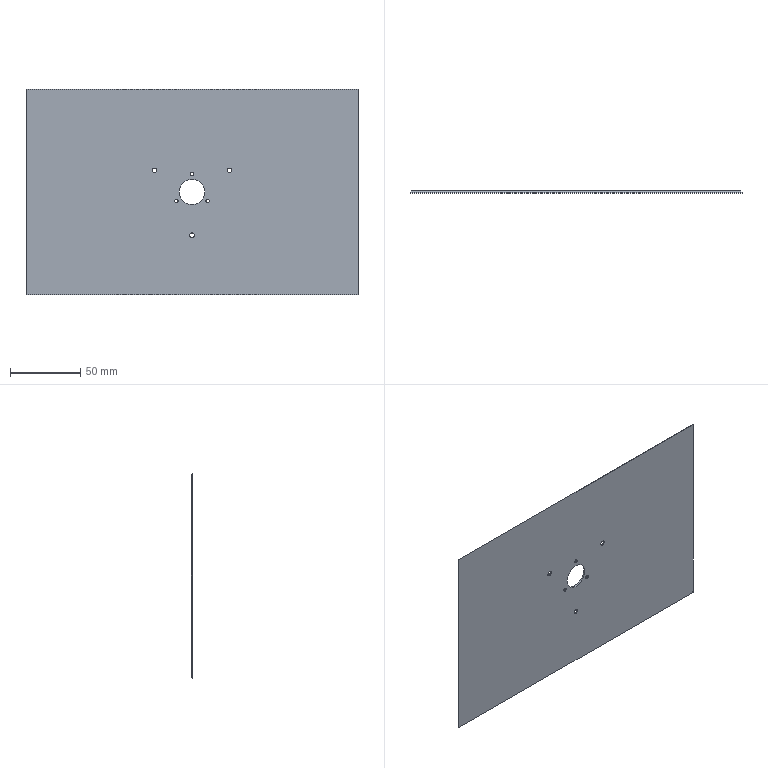Part | NX | 1 solid | 32 faces | box 236.4 x 1.2 x 146.4 mm | volume 40622 mm3 | cylinder 14 | cone 12 | plane 6 | commonest cylinder face diameters 2.5 x6 3.3 x6 18 x2
STEP:
#1=CARTESIAN_POINT('',(-117.,110.,72.));
#2=VERTEX_POINT('',#1);
#3=CARTESIAN_POINT('',(-117.,110.,-72.));
#4=VERTEX_POINT('',#3);
#5=CARTESIAN_POINT('',(-117.,110.,0.));
#6=DIRECTION('',(0.,0.,-1.));
#7=VECTOR('',#6,1000.);
#8=LINE('',#5,#7);
#9=EDGE_CURVE('',#2,#4,#8,.T.);
#10=ORIENTED_EDGE('',*,*,#9,.F.);
#11=CARTESIAN_POINT('',(117.,110.,72.));
#12=VERTEX_POINT('',#11);
#13=CARTESIAN_POINT('',(0.,110.,72.));
#14=DIRECTION('',(-1.,0.,0.));
#15=VECTOR('',#14,1000.);
#16=LINE('',#13,#15);
#17=EDGE_CURVE('',#12,#2,#16,.T.);
#18=ORIENTED_EDGE('',*,*,#17,.F.);
#19=CARTESIAN_POINT('',(117.,110.,-72.));
#20=VERTEX_POINT('',#19);
#21=CARTESIAN_POINT('',(117.,110.,0.));
#22=DIRECTION('',(0.,0.,1.));
#23=VECTOR('',#22,1000.);
#24=LINE('',#21,#23);
#25=EDGE_CURVE('',#20,#12,#24,.T.);
#26=ORIENTED_EDGE('',*,*,#25,.F.);
#27=CARTESIAN_POINT('',(0.,110.,-72.));
#28=DIRECTION('',(-1.,0.,0.));
#29=VECTOR('',#28,1000.);
#30=LINE('',#27,#29);
#31=EDGE_CURVE('',#20,#4,#30,.T.);
#32=ORIENTED_EDGE('',*,*,#31,.T.);
#33=EDGE_LOOP('',(#10,#18,#26,#32));
#34=FACE_BOUND('',#33,.T.);
#35=CARTESIAN_POINT('',(-28.945,110.,15.375));
#36=VERTEX_POINT('',#35);
#37=CARTESIAN_POINT('',(-24.315,110.,15.375));
#38=VERTEX_POINT('',#37);
#39=CARTESIAN_POINT('',(-26.63,110.,15.375));
#40=DIRECTION('',(0.,1.,0.));
#41=DIRECTION('',(1.,0.,0.));
#42=AXIS2_PLACEMENT_3D('',#39,#40,#41);
#43=CIRCLE('',#42,2.315);
#44=EDGE_CURVE('',#36,#38,#43,.T.);
#45=ORIENTED_EDGE('',*,*,#44,.F.);
#46=CARTESIAN_POINT('',(-26.63,110.,15.375));
#47=DIRECTION('',(0.,1.,0.));
#48=DIRECTION('',(1.,0.,0.));
#49=AXIS2_PLACEMENT_3D('',#46,#47,#48);
#50=CIRCLE('',#49,2.315);
#51=EDGE_CURVE('',#38,#36,#50,.T.);
#52=ORIENTED_EDGE('',*,*,#51,.F.);
#53=EDGE_LOOP('',(#45,#52));
#54=FACE_BOUND('',#53,.T.);
#55=CARTESIAN_POINT('',(24.315,110.,15.375));
#56=VERTEX_POINT('',#55);
#57=CARTESIAN_POINT('',(28.945,110.,15.375));
#58=VERTEX_POINT('',#57);
#59=CARTESIAN_POINT('',(26.63,110.,15.375));
#60=DIRECTION('',(0.,1.,0.));
#61=DIRECTION('',(1.,0.,0.));
#62=AXIS2_PLACEMENT_3D('',#59,#60,#61);
#63=CIRCLE('',#62,2.315);
#64=EDGE_CURVE('',#56,#58,#63,.T.);
#65=ORIENTED_EDGE('',*,*,#64,.F.);
#66=CARTESIAN_POINT('',(26.63,110.,15.375));
#67=DIRECTION('',(0.,1.,0.));
#68=DIRECTION('',(1.,0.,0.));
#69=AXIS2_PLACEMENT_3D('',#66,#67,#68);
#70=CIRCLE('',#69,2.315);
#71=EDGE_CURVE('',#58,#56,#70,.T.);
#72=ORIENTED_EDGE('',*,*,#71,.F.);
#73=EDGE_LOOP('',(#65,#72));
#74=FACE_BOUND('',#73,.T.);
#75=CARTESIAN_POINT('',(-2.315,110.,-30.75));
#76=VERTEX_POINT('',#75);
#77=CARTESIAN_POINT('',(2.315,110.,-30.75));
#78=VERTEX_POINT('',#77);
#79=CARTESIAN_POINT('',(0.,110.,-30.75));
#80=DIRECTION('',(0.,1.,0.));
#81=DIRECTION('',(1.,0.,0.));
#82=AXIS2_PLACEMENT_3D('',#79,#80,#81);
#83=CIRCLE('',#82,2.315);
#84=EDGE_CURVE('',#76,#78,#83,.T.);
#85=ORIENTED_EDGE('',*,*,#84,.F.);
#86=CARTESIAN_POINT('',(0.,110.,-30.75));
#87=DIRECTION('',(0.,1.,0.));
#88=DIRECTION('',(1.,0.,0.));
#89=AXIS2_PLACEMENT_3D('',#86,#87,#88);
#90=CIRCLE('',#89,2.315);
#91=EDGE_CURVE('',#78,#76,#90,.T.);
#92=ORIENTED_EDGE('',*,*,#91,.F.);
#93=EDGE_LOOP('',(#85,#92));
#94=FACE_BOUND('',#93,.T.);
#95=CARTESIAN_POINT('',(-1.7,110.,12.8));
#96=VERTEX_POINT('',#95);
#97=CARTESIAN_POINT('',(1.7,110.,12.8));
#98=VERTEX_POINT('',#97);
#99=CARTESIAN_POINT('',(0.,110.,12.8));
#100=DIRECTION('',(0.,1.,0.));
#101=DIRECTION('',(1.,0.,0.));
#102=AXIS2_PLACEMENT_3D('',#99,#100,#101);
#103=CIRCLE('',#102,1.7);
#104=EDGE_CURVE('',#96,#98,#103,.T.);
#105=ORIENTED_EDGE('',*,*,#104,.F.);
#106=CARTESIAN_POINT('',(0.,110.,12.8));
#107=DIRECTION('',(0.,1.,0.));
#108=DIRECTION('',(1.,0.,0.));
#109=AXIS2_PLACEMENT_3D('',#106,#107,#108);
#110=CIRCLE('',#109,1.7);
#111=EDGE_CURVE('',#98,#96,#110,.T.);
#112=ORIENTED_EDGE('',*,*,#111,.F.);
#113=EDGE_LOOP('',(#105,#112));
#114=FACE_BOUND('',#113,.T.);
#115=CARTESIAN_POINT('',(-9.,110.,0.));
#116=VERTEX_POINT('',#115);
#117=CARTESIAN_POINT('',(9.,110.,0.));
#118=VERTEX_POINT('',#117);
#119=CARTESIAN_POINT('',(0.,110.,0.));
#120=DIRECTION('',(0.,-1.,0.));
#121=DIRECTION('',(1.,0.,0.));
#122=AXIS2_PLACEMENT_3D('',#119,#120,#121);
#123=CIRCLE('',#122,9.);
#124=EDGE_CURVE('',#116,#118,#123,.T.);
#125=ORIENTED_EDGE('',*,*,#124,.T.);
#126=CARTESIAN_POINT('',(0.,110.,0.));
#127=DIRECTION('',(0.,-1.,0.));
#128=DIRECTION('',(1.,0.,0.));
#129=AXIS2_PLACEMENT_3D('',#126,#127,#128);
#130=CIRCLE('',#129,9.);
#131=EDGE_CURVE('',#118,#116,#130,.T.);
#132=ORIENTED_EDGE('',*,*,#131,.T.);
#133=EDGE_LOOP('',(#125,#132));
#134=FACE_BOUND('',#133,.T.);
#135=CARTESIAN_POINT('',(9.385,110.,-6.4));
#136=VERTEX_POINT('',#135);
#137=CARTESIAN_POINT('',(12.785,110.,-6.4));
#138=VERTEX_POINT('',#137);
#139=CARTESIAN_POINT('',(11.085,110.,-6.4));
#140=DIRECTION('',(0.,1.,0.));
#141=DIRECTION('',(1.,0.,0.));
#142=AXIS2_PLACEMENT_3D('',#139,#140,#141);
#143=CIRCLE('',#142,1.7);
#144=EDGE_CURVE('',#136,#138,#143,.T.);
#145=ORIENTED_EDGE('',*,*,#144,.F.);
#146=CARTESIAN_POINT('',(11.085,110.,-6.4));
#147=DIRECTION('',(0.,1.,0.));
#148=DIRECTION('',(1.,0.,0.));
#149=AXIS2_PLACEMENT_3D('',#146,#147,#148);
#150=CIRCLE('',#149,1.7);
#151=EDGE_CURVE('',#138,#136,#150,.T.);
#152=ORIENTED_EDGE('',*,*,#151,.F.);
#153=EDGE_LOOP('',(#145,#152));
#154=FACE_BOUND('',#153,.T.);
#155=CARTESIAN_POINT('',(-12.785,110.,-6.4));
#156=VERTEX_POINT('',#155);
#157=CARTESIAN_POINT('',(-9.385,110.,-6.4));
#158=VERTEX_POINT('',#157);
#159=CARTESIAN_POINT('',(-11.085,110.,-6.4));
#160=DIRECTION('',(0.,1.,0.));
#161=DIRECTION('',(1.,0.,0.));
#162=AXIS2_PLACEMENT_3D('',#159,#160,#161);
#163=CIRCLE('',#162,1.7);
#164=EDGE_CURVE('',#156,#158,#163,.T.);
#165=ORIENTED_EDGE('',*,*,#164,.F.);
#166=CARTESIAN_POINT('',(-11.085,110.,-6.4));
#167=DIRECTION('',(0.,1.,0.));
#168=DIRECTION('',(1.,0.,0.));
#169=AXIS2_PLACEMENT_3D('',#166,#167,#168);
#170=CIRCLE('',#169,1.7);
#171=EDGE_CURVE('',#158,#156,#170,.T.);
#172=ORIENTED_EDGE('',*,*,#171,.F.);
#173=EDGE_LOOP('',(#165,#172));
#174=FACE_BOUND('',#173,.T.);
#175=CARTESIAN_POINT('',(120.,110.,-75.));
#176=DIRECTION('',(0.,1.,0.));
#177=DIRECTION('',(1.,0.,0.));
#178=AXIS2_PLACEMENT_3D('',#175,#176,#177);
#179=PLANE('',#178);
#180=ADVANCED_FACE('',(#34,#54,#74,#94,#114,#134,#154,#174),#179,.T.);
#181=CARTESIAN_POINT('',(-12.335,109.74,-6.4));
#182=VERTEX_POINT('',#181);
#183=CARTESIAN_POINT('',(-9.835,109.74,-6.4));
#184=VERTEX_POINT('',#183);
#185=CARTESIAN_POINT('',(-11.085,109.74,-6.4));
#186=DIRECTION('',(0.,1.,0.));
#187=DIRECTION('',(1.,0.,0.));
#188=AXIS2_PLACEMENT_3D('',#185,#186,#187);
#189=CIRCLE('',#188,1.25);
#190=EDGE_CURVE('',#182,#184,#189,.T.);
#191=ORIENTED_EDGE('',*,*,#190,.T.);
#192=CARTESIAN_POINT('',(-9.835,108.8,-6.4));
#193=VERTEX_POINT('',#192);
#194=CARTESIAN_POINT('',(-9.835,110.,-6.4));
#195=DIRECTION('',(0.,1.,0.));
#196=VECTOR('',#195,1000.);
#197=LINE('',#194,#196);
#198=EDGE_CURVE('',#193,#184,#197,.T.);
#199=ORIENTED_EDGE('',*,*,#198,.F.);
#200=CARTESIAN_POINT('',(-12.335,108.8,-6.4));
#201=VERTEX_POINT('',#200);
#202=CARTESIAN_POINT('',(-11.085,108.8,-6.4));
#203=DIRECTION('',(0.,1.,0.));
#204=DIRECTION('',(1.,0.,0.));
#205=AXIS2_PLACEMENT_3D('',#202,#203,#204);
#206=CIRCLE('',#205,1.25);
#207=EDGE_CURVE('',#201,#193,#206,.T.);
#208=ORIENTED_EDGE('',*,*,#207,.F.);
#209=CARTESIAN_POINT('',(-12.335,110.,-6.4));
#210=DIRECTION('',(0.,1.,0.));
#211=VECTOR('',#210,1000.);
#212=LINE('',#209,#211);
#213=EDGE_CURVE('',#201,#182,#212,.T.);
#214=ORIENTED_EDGE('',*,*,#213,.T.);
#215=EDGE_LOOP('',(#191,#199,#208,#214));
#216=FACE_BOUND('',#215,.T.);
#217=CARTESIAN_POINT('',(-11.085,110.,-6.4));
#218=DIRECTION('',(0.,1.,0.));
#219=DIRECTION('',(1.,0.,0.));
#220=AXIS2_PLACEMENT_3D('',#217,#218,#219);
#221=CYLINDRICAL_SURFACE('',#220,1.25);
#222=ADVANCED_FACE('',(#216),#221,.F.);
#223=ORIENTED_EDGE('',*,*,#25,.T.);
#224=CARTESIAN_POINT('',(118.2,108.8,73.2));
#225=VERTEX_POINT('',#224);
#226=CARTESIAN_POINT('',(45.,182.,0.));
#227=DIRECTION('',(0.5774,-0.5774,0.5774));
#228=VECTOR('',#227,1000.);
#229=LINE('',#226,#228);
#230=EDGE_CURVE('',#12,#225,#229,.T.);
#231=ORIENTED_EDGE('',*,*,#230,.T.);
#232=CARTESIAN_POINT('',(118.2,108.8,-73.2));
#233=VERTEX_POINT('',#232);
#234=CARTESIAN_POINT('',(118.2,108.8,0.));
#235=DIRECTION('',(0.,0.,1.));
#236=VECTOR('',#235,1000.);
#237=LINE('',#234,#236);
#238=EDGE_CURVE('',#233,#225,#237,.T.);
#239=ORIENTED_EDGE('',*,*,#238,.F.);
#240=CARTESIAN_POINT('',(45.,182.,0.));
#241=DIRECTION('',(-0.5774,0.5774,0.5774));
#242=VECTOR('',#241,1000.);
#243=LINE('',#240,#242);
#244=EDGE_CURVE('',#233,#20,#243,.T.);
#245=ORIENTED_EDGE('',*,*,#244,.T.);
#246=EDGE_LOOP('',(#223,#231,#239,#245));
#247=FACE_BOUND('',#246,.T.);
#248=CARTESIAN_POINT('',(118.5,108.5,0.));
#249=DIRECTION('',(-0.7071,-0.7071,0.));
#250=DIRECTION('',(-0.7071,0.7071,0.));
#251=AXIS2_PLACEMENT_3D('',#248,#249,#250);
#252=PLANE('',#251);
#253=ADVANCED_FACE('',(#247),#252,.F.);
#254=CARTESIAN_POINT('',(9.835,109.74,-6.4));
#255=VERTEX_POINT('',#254);
#256=CARTESIAN_POINT('',(12.335,109.74,-6.4));
#257=VERTEX_POINT('',#256);
#258=CARTESIAN_POINT('',(11.085,109.74,-6.4));
#259=DIRECTION('',(0.,1.,0.));
#260=DIRECTION('',(1.,0.,0.));
#261=AXIS2_PLACEMENT_3D('',#258,#259,#260);
#262=CIRCLE('',#261,1.25);
#263=EDGE_CURVE('',#255,#257,#262,.T.);
#264=ORIENTED_EDGE('',*,*,#263,.T.);
#265=CARTESIAN_POINT('',(12.335,108.8,-6.4));
#266=VERTEX_POINT('',#265);
#267=CARTESIAN_POINT('',(12.335,110.,-6.4));
#268=DIRECTION('',(0.,1.,0.));
#269=VECTOR('',#268,1000.);
#270=LINE('',#267,#269);
#271=EDGE_CURVE('',#266,#257,#270,.T.);
#272=ORIENTED_EDGE('',*,*,#271,.F.);
#273=CARTESIAN_POINT('',(9.835,108.8,-6.4));
#274=VERTEX_POINT('',#273);
#275=CARTESIAN_POINT('',(11.085,108.8,-6.4));
#276=DIRECTION('',(0.,1.,0.));
#277=DIRECTION('',(1.,0.,0.));
#278=AXIS2_PLACEMENT_3D('',#275,#276,#277);
#279=CIRCLE('',#278,1.25);
#280=EDGE_CURVE('',#274,#266,#279,.T.);
#281=ORIENTED_EDGE('',*,*,#280,.F.);
#282=CARTESIAN_POINT('',(9.835,110.,-6.4));
#283=DIRECTION('',(0.,1.,0.));
#284=VECTOR('',#283,1000.);
#285=LINE('',#282,#284);
#286=EDGE_CURVE('',#274,#255,#285,.T.);
#287=ORIENTED_EDGE('',*,*,#286,.T.);
#288=EDGE_LOOP('',(#264,#272,#281,#287));
#289=FACE_BOUND('',#288,.T.);
#290=CARTESIAN_POINT('',(11.085,110.,-6.4));
#291=DIRECTION('',(0.,1.,0.));
#292=DIRECTION('',(1.,0.,0.));
#293=AXIS2_PLACEMENT_3D('',#290,#291,#292);
#294=CYLINDRICAL_SURFACE('',#293,1.25);
#295=ADVANCED_FACE('',(#289),#294,.F.);
#296=CARTESIAN_POINT('',(-1.25,109.74,12.8));
#297=VERTEX_POINT('',#296);
#298=CARTESIAN_POINT('',(1.25,109.74,12.8));
#299=VERTEX_POINT('',#298);
#300=CARTESIAN_POINT('',(0.,109.74,12.8));
#301=DIRECTION('',(0.,1.,0.));
#302=DIRECTION('',(1.,0.,0.));
#303=AXIS2_PLACEMENT_3D('',#300,#301,#302);
#304=CIRCLE('',#303,1.25);
#305=EDGE_CURVE('',#297,#299,#304,.T.);
#306=ORIENTED_EDGE('',*,*,#305,.F.);
#307=CARTESIAN_POINT('',(-1.25,109.74,12.8));
#308=DIRECTION('',(-0.866,0.5,0.));
#309=VECTOR('',#308,1000.);
#310=LINE('',#307,#309);
#311=EDGE_CURVE('',#297,#96,#310,.T.);
#312=ORIENTED_EDGE('',*,*,#311,.T.);
#313=ORIENTED_EDGE('',*,*,#104,.T.);
#314=CARTESIAN_POINT('',(1.25,109.74,12.8));
#315=DIRECTION('',(0.866,0.5,0.));
#316=VECTOR('',#315,1000.);
#317=LINE('',#314,#316);
#318=EDGE_CURVE('',#299,#98,#317,.T.);
#319=ORIENTED_EDGE('',*,*,#318,.F.);
#320=EDGE_LOOP('',(#306,#312,#313,#319));
#321=FACE_BOUND('',#320,.T.);
#322=CARTESIAN_POINT('',(0.,109.74,12.8));
#323=DIRECTION('',(0.,1.,0.));
#324=DIRECTION('',(1.,0.,0.));
#325=AXIS2_PLACEMENT_3D('',#322,#323,#324);
#326=CONICAL_SURFACE('',#325,1.25,1.047);
#327=ADVANCED_FACE('',(#321),#326,.F.);
#328=ORIENTED_EDGE('',*,*,#263,.F.);
#329=CARTESIAN_POINT('',(9.835,109.74,-6.4));
#330=DIRECTION('',(-0.866,0.5,0.));
#331=VECTOR('',#330,1000.);
#332=LINE('',#329,#331);
#333=EDGE_CURVE('',#255,#136,#332,.T.);
#334=ORIENTED_EDGE('',*,*,#333,.T.);
#335=ORIENTED_EDGE('',*,*,#144,.T.);
#336=CARTESIAN_POINT('',(12.335,109.74,-6.4));
#337=DIRECTION('',(0.866,0.5,0.));
#338=VECTOR('',#337,1000.);
#339=LINE('',#336,#338);
#340=EDGE_CURVE('',#257,#138,#339,.T.);
#341=ORIENTED_EDGE('',*,*,#340,.F.);
#342=EDGE_LOOP('',(#328,#334,#335,#341));
#343=FACE_BOUND('',#342,.T.);
#344=CARTESIAN_POINT('',(11.085,109.74,-6.4));
#345=DIRECTION('',(0.,1.,0.));
#346=DIRECTION('',(1.,0.,0.));
#347=AXIS2_PLACEMENT_3D('',#344,#345,#346);
#348=CONICAL_SURFACE('',#347,1.25,1.047);
#349=ADVANCED_FACE('',(#343),#348,.F.);
#350=ORIENTED_EDGE('',*,*,#190,.F.);
#351=CARTESIAN_POINT('',(-12.335,109.74,-6.4));
#352=DIRECTION('',(-0.866,0.5,0.));
#353=VECTOR('',#352,1000.);
#354=LINE('',#351,#353);
#355=EDGE_CURVE('',#182,#156,#354,.T.);
#356=ORIENTED_EDGE('',*,*,#355,.T.);
#357=ORIENTED_EDGE('',*,*,#164,.T.);
#358=CARTESIAN_POINT('',(-9.835,109.74,-6.4));
#359=DIRECTION('',(0.866,0.5,0.));
#360=VECTOR('',#359,1000.);
#361=LINE('',#358,#360);
#362=EDGE_CURVE('',#184,#158,#361,.T.);
#363=ORIENTED_EDGE('',*,*,#362,.F.);
#364=EDGE_LOOP('',(#350,#356,#357,#363));
#365=FACE_BOUND('',#364,.T.);
#366=CARTESIAN_POINT('',(-11.085,109.74,-6.4));
#367=DIRECTION('',(0.,1.,0.));
#368=DIRECTION('',(1.,0.,0.));
#369=AXIS2_PLACEMENT_3D('',#366,#367,#368);
#370=CONICAL_SURFACE('',#369,1.25,1.047);
#371=ADVANCED_FACE('',(#365),#370,.F.);
#372=ORIENTED_EDGE('',*,*,#17,.T.);
#373=CARTESIAN_POINT('',(-118.2,108.8,73.2));
#374=VERTEX_POINT('',#373);
#375=CARTESIAN_POINT('',(-45.,182.,0.));
#376=DIRECTION('',(0.5774,0.5774,-0.5774));
#377=VECTOR('',#376,1000.);
#378=LINE('',#375,#377);
#379=EDGE_CURVE('',#374,#2,#378,.T.);
#380=ORIENTED_EDGE('',*,*,#379,.F.);
#381=CARTESIAN_POINT('',(0.,108.8,73.2));
#382=DIRECTION('',(-1.,0.,0.));
#383=VECTOR('',#382,1000.);
#384=LINE('',#381,#383);
#385=EDGE_CURVE('',#225,#374,#384,.T.);
#386=ORIENTED_EDGE('',*,*,#385,.F.);
#387=ORIENTED_EDGE('',*,*,#230,.F.);
#388=EDGE_LOOP('',(#372,#380,#386,#387));
#389=FACE_BOUND('',#388,.T.);
#390=CARTESIAN_POINT('',(0.,108.5,73.5));
#391=DIRECTION('',(0.,-0.7071,-0.7071));
#392=DIRECTION('',(0.,-0.7071,0.7071));
#393=AXIS2_PLACEMENT_3D('',#390,#391,#392);
#394=PLANE('',#393);
#395=ADVANCED_FACE('',(#389),#394,.F.);
#396=CARTESIAN_POINT('',(24.98,109.616,15.375));
#397=VERTEX_POINT('',#396);
#398=CARTESIAN_POINT('',(28.28,109.616,15.375));
#399=VERTEX_POINT('',#398);
#400=CARTESIAN_POINT('',(26.63,109.616,15.375));
#401=DIRECTION('',(0.,1.,0.));
#402=DIRECTION('',(1.,0.,0.));
#403=AXIS2_PLACEMENT_3D('',#400,#401,#402);
#404=CIRCLE('',#403,1.65);
#405=EDGE_CURVE('',#397,#399,#404,.T.);
#406=ORIENTED_EDGE('',*,*,#405,.T.);
#407=CARTESIAN_POINT('',(28.28,108.8,15.375));
#408=VERTEX_POINT('',#407);
#409=CARTESIAN_POINT('',(28.28,110.,15.375));
#410=DIRECTION('',(0.,1.,0.));
#411=VECTOR('',#410,1000.);
#412=LINE('',#409,#411);
#413=EDGE_CURVE('',#408,#399,#412,.T.);
#414=ORIENTED_EDGE('',*,*,#413,.F.);
#415=CARTESIAN_POINT('',(24.98,108.8,15.375));
#416=VERTEX_POINT('',#415);
#417=CARTESIAN_POINT('',(26.63,108.8,15.375));
#418=DIRECTION('',(0.,1.,0.));
#419=DIRECTION('',(1.,0.,0.));
#420=AXIS2_PLACEMENT_3D('',#417,#418,#419);
#421=CIRCLE('',#420,1.65);
#422=EDGE_CURVE('',#416,#408,#421,.T.);
#423=ORIENTED_EDGE('',*,*,#422,.F.);
#424=CARTESIAN_POINT('',(24.98,110.,15.375));
#425=DIRECTION('',(0.,1.,0.));
#426=VECTOR('',#425,1000.);
#427=LINE('',#424,#426);
#428=EDGE_CURVE('',#416,#397,#427,.T.);
#429=ORIENTED_EDGE('',*,*,#428,.T.);
#430=EDGE_LOOP('',(#406,#414,#423,#429));
#431=FACE_BOUND('',#430,.T.);
#432=CARTESIAN_POINT('',(26.63,110.,15.375));
#433=DIRECTION('',(0.,1.,0.));
#434=DIRECTION('',(1.,0.,0.));
#435=AXIS2_PLACEMENT_3D('',#432,#433,#434);
#436=CYLINDRICAL_SURFACE('',#435,1.65);
#437=ADVANCED_FACE('',(#431),#436,.F.);
#438=ORIENTED_EDGE('',*,*,#405,.F.);
#439=CARTESIAN_POINT('',(24.98,109.616,15.375));
#440=DIRECTION('',(-0.866,0.5,0.));
#441=VECTOR('',#440,1000.);
#442=LINE('',#439,#441);
#443=EDGE_CURVE('',#397,#56,#442,.T.);
#444=ORIENTED_EDGE('',*,*,#443,.T.);
#445=ORIENTED_EDGE('',*,*,#64,.T.);
#446=CARTESIAN_POINT('',(28.28,109.616,15.375));
#447=DIRECTION('',(0.866,0.5,0.));
#448=VECTOR('',#447,1000.);
#449=LINE('',#446,#448);
#450=EDGE_CURVE('',#399,#58,#449,.T.);
#451=ORIENTED_EDGE('',*,*,#450,.F.);
#452=EDGE_LOOP('',(#438,#444,#445,#451));
#453=FACE_BOUND('',#452,.T.);
#454=CARTESIAN_POINT('',(26.63,109.616,15.375));
#455=DIRECTION('',(0.,1.,0.));
#456=DIRECTION('',(1.,0.,0.));
#457=AXIS2_PLACEMENT_3D('',#454,#455,#456);
#458=CONICAL_SURFACE('',#457,1.65,1.047);
#459=ADVANCED_FACE('',(#453),#458,.F.);
#460=ORIENTED_EDGE('',*,*,#9,.T.);
#461=CARTESIAN_POINT('',(-118.2,108.8,-73.2));
#462=VERTEX_POINT('',#461);
#463=CARTESIAN_POINT('',(-45.,182.,0.));
#464=DIRECTION('',(-0.5774,-0.5774,-0.5774));
#465=VECTOR('',#464,1000.);
#466=LINE('',#463,#465);
#467=EDGE_CURVE('',#4,#462,#466,.T.);
#468=ORIENTED_EDGE('',*,*,#467,.T.);
#469=CARTESIAN_POINT('',(-118.2,108.8,0.));
#470=DIRECTION('',(0.,0.,-1.));
#471=VECTOR('',#470,1000.);
#472=LINE('',#469,#471);
#473=EDGE_CURVE('',#374,#462,#472,.T.);
#474=ORIENTED_EDGE('',*,*,#473,.F.);
#475=ORIENTED_EDGE('',*,*,#379,.T.);
#476=EDGE_LOOP('',(#460,#468,#474,#475));
#477=FACE_BOUND('',#476,.T.);
#478=CARTESIAN_POINT('',(-118.5,108.5,0.));
#479=DIRECTION('',(0.7071,-0.7071,0.));
#480=DIRECTION('',(0.,0.,-1.));
#481=AXIS2_PLACEMENT_3D('',#478,#479,#480);
#482=PLANE('',#481);
#483=ADVANCED_FACE('',(#477),#482,.F.);
#484=CARTESIAN_POINT('',(-1.65,109.616,-30.75));
#485=VERTEX_POINT('',#484);
#486=CARTESIAN_POINT('',(1.65,109.616,-30.75));
#487=VERTEX_POINT('',#486);
#488=CARTESIAN_POINT('',(0.,109.616,-30.75));
#489=DIRECTION('',(0.,1.,0.));
#490=DIRECTION('',(1.,0.,0.));
#491=AXIS2_PLACEMENT_3D('',#488,#489,#490);
#492=CIRCLE('',#491,1.65);
#493=EDGE_CURVE('',#485,#487,#492,.T.);
#494=ORIENTED_EDGE('',*,*,#493,.F.);
#495=CARTESIAN_POINT('',(-1.65,109.616,-30.75));
#496=DIRECTION('',(-0.866,0.5,0.));
#497=VECTOR('',#496,1000.);
#498=LINE('',#495,#497);
#499=EDGE_CURVE('',#485,#76,#498,.T.);
#500=ORIENTED_EDGE('',*,*,#499,.T.);
#501=ORIENTED_EDGE('',*,*,#84,.T.);
#502=CARTESIAN_POINT('',(1.65,109.616,-30.75));
#503=DIRECTION('',(0.866,0.5,0.));
#504=VECTOR('',#503,1000.);
#505=LINE('',#502,#504);
#506=EDGE_CURVE('',#487,#78,#505,.T.);
#507=ORIENTED_EDGE('',*,*,#506,.F.);
#508=EDGE_LOOP('',(#494,#500,#501,#507));
#509=FACE_BOUND('',#508,.T.);
#510=CARTESIAN_POINT('',(0.,109.616,-30.75));
#511=DIRECTION('',(0.,1.,0.));
#512=DIRECTION('',(1.,0.,0.));
#513=AXIS2_PLACEMENT_3D('',#510,#511,#512);
#514=CONICAL_SURFACE('',#513,1.65,1.047);
#515=ADVANCED_FACE('',(#509),#514,.F.);
#516=ORIENTED_EDGE('',*,*,#238,.T.);
#517=ORIENTED_EDGE('',*,*,#385,.T.);
#518=ORIENTED_EDGE('',*,*,#473,.T.);
#519=CARTESIAN_POINT('',(0.,108.8,-73.2));
#520=DIRECTION('',(-1.,0.,0.));
#521=VECTOR('',#520,1000.);
#522=LINE('',#519,#521);
#523=EDGE_CURVE('',#233,#462,#522,.T.);
#524=ORIENTED_EDGE('',*,*,#523,.F.);
#525=EDGE_LOOP('',(#516,#517,#518,#524));
#526=FACE_BOUND('',#525,.T.);
#527=ORIENTED_EDGE('',*,*,#422,.T.);
#528=CARTESIAN_POINT('',(26.63,108.8,15.375));
#529=DIRECTION('',(0.,1.,0.));
#530=DIRECTION('',(1.,0.,0.));
#531=AXIS2_PLACEMENT_3D('',#528,#529,#530);
#532=CIRCLE('',#531,1.65);
#533=EDGE_CURVE('',#408,#416,#532,.T.);
#534=ORIENTED_EDGE('',*,*,#533,.T.);
#535=EDGE_LOOP('',(#527,#534));
#536=FACE_BOUND('',#535,.T.);
#537=CARTESIAN_POINT('',(-1.65,108.8,-30.75));
#538=VERTEX_POINT('',#537);
#539=CARTESIAN_POINT('',(1.65,108.8,-30.75));
#540=VERTEX_POINT('',#539);
#541=CARTESIAN_POINT('',(0.,108.8,-30.75));
#542=DIRECTION('',(0.,1.,0.));
#543=DIRECTION('',(1.,0.,0.));
#544=AXIS2_PLACEMENT_3D('',#541,#542,#543);
#545=CIRCLE('',#544,1.65);
#546=EDGE_CURVE('',#538,#540,#545,.T.);
#547=ORIENTED_EDGE('',*,*,#546,.T.);
#548=CARTESIAN_POINT('',(0.,108.8,-30.75));
#549=DIRECTION('',(0.,1.,0.));
#550=DIRECTION('',(1.,0.,0.));
#551=AXIS2_PLACEMENT_3D('',#548,#549,#550);
#552=CIRCLE('',#551,1.65);
#553=EDGE_CURVE('',#540,#538,#552,.T.);
#554=ORIENTED_EDGE('',*,*,#553,.T.);
#555=EDGE_LOOP('',(#547,#554));
#556=FACE_BOUND('',#555,.T.);
#557=ORIENTED_EDGE('',*,*,#207,.T.);
#558=CARTESIAN_POINT('',(-11.085,108.8,-6.4));
#559=DIRECTION('',(0.,1.,0.));
#560=DIRECTION('',(1.,0.,0.));
#561=AXIS2_PLACEMENT_3D('',#558,#559,#560);
#562=CIRCLE('',#561,1.25);
#563=EDGE_CURVE('',#193,#201,#562,.T.);
#564=ORIENTED_EDGE('',*,*,#563,.T.);
#565=EDGE_LOOP('',(#557,#564));
#566=FACE_BOUND('',#565,.T.);
#567=CARTESIAN_POINT('',(-1.25,108.8,12.8));
#568=VERTEX_POINT('',#567);
#569=CARTESIAN_POINT('',(1.25,108.8,12.8));
#570=VERTEX_POINT('',#569);
#571=CARTESIAN_POINT('',(0.,108.8,12.8));
#572=DIRECTION('',(0.,1.,0.));
#573=DIRECTION('',(1.,0.,0.));
#574=AXIS2_PLACEMENT_3D('',#571,#572,#573);
#575=CIRCLE('',#574,1.25);
#576=EDGE_CURVE('',#568,#570,#575,.T.);
#577=ORIENTED_EDGE('',*,*,#576,.T.);
#578=CARTESIAN_POINT('',(0.,108.8,12.8));
#579=DIRECTION('',(0.,1.,0.));
#580=DIRECTION('',(1.,0.,0.));
#581=AXIS2_PLACEMENT_3D('',#578,#579,#580);
#582=CIRCLE('',#581,1.25);
#583=EDGE_CURVE('',#570,#568,#582,.T.);
#584=ORIENTED_EDGE('',*,*,#583,.T.);
#585=EDGE_LOOP('',(#577,#584));
#586=FACE_BOUND('',#585,.T.);
#587=ORIENTED_EDGE('',*,*,#280,.T.);
#588=CARTESIAN_POINT('',(11.085,108.8,-6.4));
#589=DIRECTION('',(0.,1.,0.));
#590=DIRECTION('',(1.,0.,0.));
#591=AXIS2_PLACEMENT_3D('',#588,#589,#590);
#592=CIRCLE('',#591,1.25);
#593=EDGE_CURVE('',#266,#274,#592,.T.);
#594=ORIENTED_EDGE('',*,*,#593,.T.);
#595=EDGE_LOOP('',(#587,#594));
#596=FACE_BOUND('',#595,.T.);
#597=CARTESIAN_POINT('',(-9.,108.8,0.));
#598=VERTEX_POINT('',#597);
#599=CARTESIAN_POINT('',(9.,108.8,0.));
#600=VERTEX_POINT('',#599);
#601=CARTESIAN_POINT('',(0.,108.8,0.));
#602=DIRECTION('',(0.,-1.,0.));
#603=DIRECTION('',(1.,0.,0.));
#604=AXIS2_PLACEMENT_3D('',#601,#602,#603);
#605=CIRCLE('',#604,9.);
#606=EDGE_CURVE('',#598,#600,#605,.T.);
#607=ORIENTED_EDGE('',*,*,#606,.F.);
#608=CARTESIAN_POINT('',(0.,108.8,0.));
#609=DIRECTION('',(0.,-1.,0.));
#610=DIRECTION('',(1.,0.,0.));
#611=AXIS2_PLACEMENT_3D('',#608,#609,#610);
#612=CIRCLE('',#611,9.);
#613=EDGE_CURVE('',#600,#598,#612,.T.);
#614=ORIENTED_EDGE('',*,*,#613,.F.);
#615=EDGE_LOOP('',(#607,#614));
#616=FACE_BOUND('',#615,.T.);
#617=CARTESIAN_POINT('',(-28.28,108.8,15.375));
#618=VERTEX_POINT('',#617);
#619=CARTESIAN_POINT('',(-24.98,108.8,15.375));
#620=VERTEX_POINT('',#619);
#621=CARTESIAN_POINT('',(-26.63,108.8,15.375));
#622=DIRECTION('',(0.,1.,0.));
#623=DIRECTION('',(1.,0.,0.));
#624=AXIS2_PLACEMENT_3D('',#621,#622,#623);
#625=CIRCLE('',#624,1.65);
#626=EDGE_CURVE('',#618,#620,#625,.T.);
#627=ORIENTED_EDGE('',*,*,#626,.T.);
#628=CARTESIAN_POINT('',(-26.63,108.8,15.375));
#629=DIRECTION('',(0.,1.,0.));
#630=DIRECTION('',(1.,0.,0.));
#631=AXIS2_PLACEMENT_3D('',#628,#629,#630);
#632=CIRCLE('',#631,1.65);
#633=EDGE_CURVE('',#620,#618,#632,.T.);
#634=ORIENTED_EDGE('',*,*,#633,.T.);
#635=EDGE_LOOP('',(#627,#634));
#636=FACE_BOUND('',#635,.T.);
#637=CARTESIAN_POINT('',(120.,108.8,-75.));
#638=DIRECTION('',(0.,1.,0.));
#639=DIRECTION('',(1.,0.,0.));
#640=AXIS2_PLACEMENT_3D('',#637,#638,#639);
#641=PLANE('',#640);
#642=ADVANCED_FACE('',(#526,#536,#556,#566,#586,#596,#616,#636),#641,.F.);
#643=CARTESIAN_POINT('',(-28.28,109.616,15.375));
#644=VERTEX_POINT('',#643);
#645=CARTESIAN_POINT('',(-24.98,109.616,15.375));
#646=VERTEX_POINT('',#645);
#647=CARTESIAN_POINT('',(-26.63,109.616,15.375));
#648=DIRECTION('',(0.,1.,0.));
#649=DIRECTION('',(1.,0.,0.));
#650=AXIS2_PLACEMENT_3D('',#647,#648,#649);
#651=CIRCLE('',#650,1.65);
#652=EDGE_CURVE('',#644,#646,#651,.T.);
#653=ORIENTED_EDGE('',*,*,#652,.T.);
#654=CARTESIAN_POINT('',(-24.98,110.,15.375));
#655=DIRECTION('',(0.,1.,0.));
#656=VECTOR('',#655,1000.);
#657=LINE('',#654,#656);
#658=EDGE_CURVE('',#620,#646,#657,.T.);
#659=ORIENTED_EDGE('',*,*,#658,.F.);
#660=ORIENTED_EDGE('',*,*,#626,.F.);
#661=CARTESIAN_POINT('',(-28.28,110.,15.375));
#662=DIRECTION('',(0.,1.,0.));
#663=VECTOR('',#662,1000.);
#664=LINE('',#661,#663);
#665=EDGE_CURVE('',#618,#644,#664,.T.);
#666=ORIENTED_EDGE('',*,*,#665,.T.);
#667=EDGE_LOOP('',(#653,#659,#660,#666));
#668=FACE_BOUND('',#667,.T.);
#669=CARTESIAN_POINT('',(-26.63,110.,15.375));
#670=DIRECTION('',(0.,1.,0.));
#671=DIRECTION('',(1.,0.,0.));
#672=AXIS2_PLACEMENT_3D('',#669,#670,#671);
#673=CYLINDRICAL_SURFACE('',#672,1.65);
#674=ADVANCED_FACE('',(#668),#673,.F.);
#675=ORIENTED_EDGE('',*,*,#31,.F.);
#676=ORIENTED_EDGE('',*,*,#244,.F.);
#677=ORIENTED_EDGE('',*,*,#523,.T.);
#678=ORIENTED_EDGE('',*,*,#467,.F.);
#679=EDGE_LOOP('',(#675,#676,#677,#678));
#680=FACE_BOUND('',#679,.T.);
#681=CARTESIAN_POINT('',(0.,108.5,-73.5));
#682=DIRECTION('',(0.,0.7071,-0.7071));
#683=DIRECTION('',(-1.,0.,0.));
#684=AXIS2_PLACEMENT_3D('',#681,#682,#683);
#685=PLANE('',#684);
#686=ADVANCED_FACE('',(#680),#685,.T.);
#687=ORIENTED_EDGE('',*,*,#606,.T.);
#688=CARTESIAN_POINT('',(9.,110.,0.));
#689=DIRECTION('',(0.,-1.,0.));
#690=VECTOR('',#689,1000.);
#691=LINE('',#688,#690);
#692=EDGE_CURVE('',#118,#600,#691,.T.);
#693=ORIENTED_EDGE('',*,*,#692,.F.);
#694=ORIENTED_EDGE('',*,*,#124,.F.);
#695=CARTESIAN_POINT('',(-9.,110.,0.));
#696=DIRECTION('',(0.,-1.,0.));
#697=VECTOR('',#696,1000.);
#698=LINE('',#695,#697);
#699=EDGE_CURVE('',#116,#598,#698,.T.);
#700=ORIENTED_EDGE('',*,*,#699,.T.);
#701=EDGE_LOOP('',(#687,#693,#694,#700));
#702=FACE_BOUND('',#701,.T.);
#703=CARTESIAN_POINT('',(0.,110.,0.));
#704=DIRECTION('',(0.,-1.,0.));
#705=DIRECTION('',(1.,0.,0.));
#706=AXIS2_PLACEMENT_3D('',#703,#704,#705);
#707=CYLINDRICAL_SURFACE('',#706,9.);
#708=ADVANCED_FACE('',(#702),#707,.F.);
#709=ORIENTED_EDGE('',*,*,#305,.T.);
#710=CARTESIAN_POINT('',(1.25,110.,12.8));
#711=DIRECTION('',(0.,1.,0.));
#712=VECTOR('',#711,1000.);
#713=LINE('',#710,#712);
#714=EDGE_CURVE('',#570,#299,#713,.T.);
#715=ORIENTED_EDGE('',*,*,#714,.F.);
#716=ORIENTED_EDGE('',*,*,#576,.F.);
#717=CARTESIAN_POINT('',(-1.25,110.,12.8));
#718=DIRECTION('',(0.,1.,0.));
#719=VECTOR('',#718,1000.);
#720=LINE('',#717,#719);
#721=EDGE_CURVE('',#568,#297,#720,.T.);
#722=ORIENTED_EDGE('',*,*,#721,.T.);
#723=EDGE_LOOP('',(#709,#715,#716,#722));
#724=FACE_BOUND('',#723,.T.);
#725=CARTESIAN_POINT('',(0.,110.,12.8));
#726=DIRECTION('',(0.,1.,0.));
#727=DIRECTION('',(1.,0.,0.));
#728=AXIS2_PLACEMENT_3D('',#725,#726,#727);
#729=CYLINDRICAL_SURFACE('',#728,1.25);
#730=ADVANCED_FACE('',(#724),#729,.F.);
#731=ORIENTED_EDGE('',*,*,#652,.F.);
#732=CARTESIAN_POINT('',(-28.28,109.616,15.375));
#733=DIRECTION('',(-0.866,0.5,0.));
#734=VECTOR('',#733,1000.);
#735=LINE('',#732,#734);
#736=EDGE_CURVE('',#644,#36,#735,.T.);
#737=ORIENTED_EDGE('',*,*,#736,.T.);
#738=ORIENTED_EDGE('',*,*,#44,.T.);
#739=CARTESIAN_POINT('',(-24.98,109.616,15.375));
#740=DIRECTION('',(0.866,0.5,0.));
#741=VECTOR('',#740,1000.);
#742=LINE('',#739,#741);
#743=EDGE_CURVE('',#646,#38,#742,.T.);
#744=ORIENTED_EDGE('',*,*,#743,.F.);
#745=EDGE_LOOP('',(#731,#737,#738,#744));
#746=FACE_BOUND('',#745,.T.);
#747=CARTESIAN_POINT('',(-26.63,109.616,15.375));
#748=DIRECTION('',(0.,1.,0.));
#749=DIRECTION('',(1.,0.,0.));
#750=AXIS2_PLACEMENT_3D('',#747,#748,#749);
#751=CONICAL_SURFACE('',#750,1.65,1.047);
#752=ADVANCED_FACE('',(#746),#751,.F.);
#753=ORIENTED_EDGE('',*,*,#493,.T.);
#754=CARTESIAN_POINT('',(1.65,110.,-30.75));
#755=DIRECTION('',(0.,1.,0.));
#756=VECTOR('',#755,1000.);
#757=LINE('',#754,#756);
#758=EDGE_CURVE('',#540,#487,#757,.T.);
#759=ORIENTED_EDGE('',*,*,#758,.F.);
#760=ORIENTED_EDGE('',*,*,#546,.F.);
#761=CARTESIAN_POINT('',(-1.65,110.,-30.75));
#762=DIRECTION('',(0.,1.,0.));
#763=VECTOR('',#762,1000.);
#764=LINE('',#761,#763);
#765=EDGE_CURVE('',#538,#485,#764,.T.);
#766=ORIENTED_EDGE('',*,*,#765,.T.);
#767=EDGE_LOOP('',(#753,#759,#760,#766));
#768=FACE_BOUND('',#767,.T.);
#769=CARTESIAN_POINT('',(0.,110.,-30.75));
#770=DIRECTION('',(0.,1.,0.));
#771=DIRECTION('',(1.,0.,0.));
#772=AXIS2_PLACEMENT_3D('',#769,#770,#771);
#773=CYLINDRICAL_SURFACE('',#772,1.65);
#774=ADVANCED_FACE('',(#768),#773,.F.);
#775=ORIENTED_EDGE('',*,*,#362,.T.);
#776=ORIENTED_EDGE('',*,*,#171,.T.);
#777=ORIENTED_EDGE('',*,*,#355,.F.);
#778=CARTESIAN_POINT('',(-11.085,109.74,-6.4));
#779=DIRECTION('',(0.,1.,0.));
#780=DIRECTION('',(1.,0.,0.));
#781=AXIS2_PLACEMENT_3D('',#778,#779,#780);
#782=CIRCLE('',#781,1.25);
#783=EDGE_CURVE('',#184,#182,#782,.T.);
#784=ORIENTED_EDGE('',*,*,#783,.F.);
#785=EDGE_LOOP('',(#775,#776,#777,#784));
#786=FACE_BOUND('',#785,.T.);
#787=CARTESIAN_POINT('',(-11.085,109.74,-6.4));
#788=DIRECTION('',(0.,1.,0.));
#789=DIRECTION('',(1.,0.,0.));
#790=AXIS2_PLACEMENT_3D('',#787,#788,#789);
#791=CONICAL_SURFACE('',#790,1.25,1.047);
#792=ADVANCED_FACE('',(#786),#791,.F.);
#793=ORIENTED_EDGE('',*,*,#758,.T.);
#794=CARTESIAN_POINT('',(0.,109.616,-30.75));
#795=DIRECTION('',(0.,1.,0.));
#796=DIRECTION('',(1.,0.,0.));
#797=AXIS2_PLACEMENT_3D('',#794,#795,#796);
#798=CIRCLE('',#797,1.65);
#799=EDGE_CURVE('',#487,#485,#798,.T.);
#800=ORIENTED_EDGE('',*,*,#799,.T.);
#801=ORIENTED_EDGE('',*,*,#765,.F.);
#802=ORIENTED_EDGE('',*,*,#553,.F.);
#803=EDGE_LOOP('',(#793,#800,#801,#802));
#804=FACE_BOUND('',#803,.T.);
#805=CARTESIAN_POINT('',(0.,110.,-30.75));
#806=DIRECTION('',(0.,1.,0.));
#807=DIRECTION('',(1.,0.,0.));
#808=AXIS2_PLACEMENT_3D('',#805,#806,#807);
#809=CYLINDRICAL_SURFACE('',#808,1.65);
#810=ADVANCED_FACE('',(#804),#809,.F.);
#811=ORIENTED_EDGE('',*,*,#450,.T.);
#812=ORIENTED_EDGE('',*,*,#71,.T.);
#813=ORIENTED_EDGE('',*,*,#443,.F.);
#814=CARTESIAN_POINT('',(26.63,109.616,15.375));
#815=DIRECTION('',(0.,1.,0.));
#816=DIRECTION('',(1.,0.,0.));
#817=AXIS2_PLACEMENT_3D('',#814,#815,#816);
#818=CIRCLE('',#817,1.65);
#819=EDGE_CURVE('',#399,#397,#818,.T.);
#820=ORIENTED_EDGE('',*,*,#819,.F.);
#821=EDGE_LOOP('',(#811,#812,#813,#820));
#822=FACE_BOUND('',#821,.T.);
#823=CARTESIAN_POINT('',(26.63,109.616,15.375));
#824=DIRECTION('',(0.,1.,0.));
#825=DIRECTION('',(1.,0.,0.));
#826=AXIS2_PLACEMENT_3D('',#823,#824,#825);
#827=CONICAL_SURFACE('',#826,1.65,1.047);
#828=ADVANCED_FACE('',(#822),#827,.F.);
#829=ORIENTED_EDGE('',*,*,#658,.T.);
#830=CARTESIAN_POINT('',(-26.63,109.616,15.375));
#831=DIRECTION('',(0.,1.,0.));
#832=DIRECTION('',(1.,0.,0.));
#833=AXIS2_PLACEMENT_3D('',#830,#831,#832);
#834=CIRCLE('',#833,1.65);
#835=EDGE_CURVE('',#646,#644,#834,.T.);
#836=ORIENTED_EDGE('',*,*,#835,.T.);
#837=ORIENTED_EDGE('',*,*,#665,.F.);
#838=ORIENTED_EDGE('',*,*,#633,.F.);
#839=EDGE_LOOP('',(#829,#836,#837,#838));
#840=FACE_BOUND('',#839,.T.);
#841=CARTESIAN_POINT('',(-26.63,110.,15.375));
#842=DIRECTION('',(0.,1.,0.));
#843=DIRECTION('',(1.,0.,0.));
#844=AXIS2_PLACEMENT_3D('',#841,#842,#843);
#845=CYLINDRICAL_SURFACE('',#844,1.65);
#846=ADVANCED_FACE('',(#840),#845,.F.);
#847=ORIENTED_EDGE('',*,*,#318,.T.);
#848=ORIENTED_EDGE('',*,*,#111,.T.);
#849=ORIENTED_EDGE('',*,*,#311,.F.);
#850=CARTESIAN_POINT('',(0.,109.74,12.8));
#851=DIRECTION('',(0.,1.,0.));
#852=DIRECTION('',(1.,0.,0.));
#853=AXIS2_PLACEMENT_3D('',#850,#851,#852);
#854=CIRCLE('',#853,1.25);
#855=EDGE_CURVE('',#299,#297,#854,.T.);
#856=ORIENTED_EDGE('',*,*,#855,.F.);
#857=EDGE_LOOP('',(#847,#848,#849,#856));
#858=FACE_BOUND('',#857,.T.);
#859=CARTESIAN_POINT('',(0.,109.74,12.8));
#860=DIRECTION('',(0.,1.,0.));
#861=DIRECTION('',(1.,0.,0.));
#862=AXIS2_PLACEMENT_3D('',#859,#860,#861);
#863=CONICAL_SURFACE('',#862,1.25,1.047);
#864=ADVANCED_FACE('',(#858),#863,.F.);
#865=ORIENTED_EDGE('',*,*,#506,.T.);
#866=ORIENTED_EDGE('',*,*,#91,.T.);
#867=ORIENTED_EDGE('',*,*,#499,.F.);
#868=ORIENTED_EDGE('',*,*,#799,.F.);
#869=EDGE_LOOP('',(#865,#866,#867,#868));
#870=FACE_BOUND('',#869,.T.);
#871=CARTESIAN_POINT('',(0.,109.616,-30.75));
#872=DIRECTION('',(0.,1.,0.));
#873=DIRECTION('',(1.,0.,0.));
#874=AXIS2_PLACEMENT_3D('',#871,#872,#873);
#875=CONICAL_SURFACE('',#874,1.65,1.047);
#876=ADVANCED_FACE('',(#870),#875,.F.);
#877=ORIENTED_EDGE('',*,*,#413,.T.);
#878=ORIENTED_EDGE('',*,*,#819,.T.);
#879=ORIENTED_EDGE('',*,*,#428,.F.);
#880=ORIENTED_EDGE('',*,*,#533,.F.);
#881=EDGE_LOOP('',(#877,#878,#879,#880));
#882=FACE_BOUND('',#881,.T.);
#883=CARTESIAN_POINT('',(26.63,110.,15.375));
#884=DIRECTION('',(0.,1.,0.));
#885=DIRECTION('',(1.,0.,0.));
#886=AXIS2_PLACEMENT_3D('',#883,#884,#885);
#887=CYLINDRICAL_SURFACE('',#886,1.65);
#888=ADVANCED_FACE('',(#882),#887,.F.);
#889=ORIENTED_EDGE('',*,*,#743,.T.);
#890=ORIENTED_EDGE('',*,*,#51,.T.);
#891=ORIENTED_EDGE('',*,*,#736,.F.);
#892=ORIENTED_EDGE('',*,*,#835,.F.);
#893=EDGE_LOOP('',(#889,#890,#891,#892));
#894=FACE_BOUND('',#893,.T.);
#895=CARTESIAN_POINT('',(-26.63,109.616,15.375));
#896=DIRECTION('',(0.,1.,0.));
#897=DIRECTION('',(1.,0.,0.));
#898=AXIS2_PLACEMENT_3D('',#895,#896,#897);
#899=CONICAL_SURFACE('',#898,1.65,1.047);
#900=ADVANCED_FACE('',(#894),#899,.F.);
#901=ORIENTED_EDGE('',*,*,#714,.T.);
#902=ORIENTED_EDGE('',*,*,#855,.T.);
#903=ORIENTED_EDGE('',*,*,#721,.F.);
#904=ORIENTED_EDGE('',*,*,#583,.F.);
#905=EDGE_LOOP('',(#901,#902,#903,#904));
#906=FACE_BOUND('',#905,.T.);
#907=CARTESIAN_POINT('',(0.,110.,12.8));
#908=DIRECTION('',(0.,1.,0.));
#909=DIRECTION('',(1.,0.,0.));
#910=AXIS2_PLACEMENT_3D('',#907,#908,#909);
#911=CYLINDRICAL_SURFACE('',#910,1.25);
#912=ADVANCED_FACE('',(#906),#911,.F.);
#913=ORIENTED_EDGE('',*,*,#271,.T.);
#914=CARTESIAN_POINT('',(11.085,109.74,-6.4));
#915=DIRECTION('',(0.,1.,0.));
#916=DIRECTION('',(1.,0.,0.));
#917=AXIS2_PLACEMENT_3D('',#914,#915,#916);
#918=CIRCLE('',#917,1.25);
#919=EDGE_CURVE('',#257,#255,#918,.T.);
#920=ORIENTED_EDGE('',*,*,#919,.T.);
#921=ORIENTED_EDGE('',*,*,#286,.F.);
#922=ORIENTED_EDGE('',*,*,#593,.F.);
#923=EDGE_LOOP('',(#913,#920,#921,#922));
#924=FACE_BOUND('',#923,.T.);
#925=CARTESIAN_POINT('',(11.085,110.,-6.4));
#926=DIRECTION('',(0.,1.,0.));
#927=DIRECTION('',(1.,0.,0.));
#928=AXIS2_PLACEMENT_3D('',#925,#926,#927);
#929=CYLINDRICAL_SURFACE('',#928,1.25);
#930=ADVANCED_FACE('',(#924),#929,.F.);
#931=ORIENTED_EDGE('',*,*,#198,.T.);
#932=ORIENTED_EDGE('',*,*,#783,.T.);
#933=ORIENTED_EDGE('',*,*,#213,.F.);
#934=ORIENTED_EDGE('',*,*,#563,.F.);
#935=EDGE_LOOP('',(#931,#932,#933,#934));
#936=FACE_BOUND('',#935,.T.);
#937=CARTESIAN_POINT('',(-11.085,110.,-6.4));
#938=DIRECTION('',(0.,1.,0.));
#939=DIRECTION('',(1.,0.,0.));
#940=AXIS2_PLACEMENT_3D('',#937,#938,#939);
#941=CYLINDRICAL_SURFACE('',#940,1.25);
#942=ADVANCED_FACE('',(#936),#941,.F.);
#943=ORIENTED_EDGE('',*,*,#692,.T.);
#944=ORIENTED_EDGE('',*,*,#613,.T.);
#945=ORIENTED_EDGE('',*,*,#699,.F.);
#946=ORIENTED_EDGE('',*,*,#131,.F.);
#947=EDGE_LOOP('',(#943,#944,#945,#946));
#948=FACE_BOUND('',#947,.T.);
#949=CARTESIAN_POINT('',(0.,110.,0.));
#950=DIRECTION('',(0.,-1.,0.));
#951=DIRECTION('',(1.,0.,0.));
#952=AXIS2_PLACEMENT_3D('',#949,#950,#951);
#953=CYLINDRICAL_SURFACE('',#952,9.);
#954=ADVANCED_FACE('',(#948),#953,.F.);
#955=ORIENTED_EDGE('',*,*,#340,.T.);
#956=ORIENTED_EDGE('',*,*,#151,.T.);
#957=ORIENTED_EDGE('',*,*,#333,.F.);
#958=ORIENTED_EDGE('',*,*,#919,.F.);
#959=EDGE_LOOP('',(#955,#956,#957,#958));
#960=FACE_BOUND('',#959,.T.);
#961=CARTESIAN_POINT('',(11.085,109.74,-6.4));
#962=DIRECTION('',(0.,1.,0.));
#963=DIRECTION('',(1.,0.,0.));
#964=AXIS2_PLACEMENT_3D('',#961,#962,#963);
#965=CONICAL_SURFACE('',#964,1.25,1.047);
#966=ADVANCED_FACE('',(#960),#965,.F.);
#967=CLOSED_SHELL('',(#180,#222,#253,#295,#327,#349,#371,#395,#437,#459,#483,#515,#642,#674,#686,#708,#730,#752,#774,#792,#810,#828,#846,#864,#876,#888,#900,#912,#930,#942,#954,#966));
#968=MANIFOLD_SOLID_BREP('',#967);
#969=(LENGTH_UNIT()NAMED_UNIT(*)SI_UNIT(.MILLI.,.METRE.));
#970=UNCERTAINTY_MEASURE_WITH_UNIT(LENGTH_MEASURE(0.00001),#969,'','');
#971=(NAMED_UNIT(*)PLANE_ANGLE_UNIT()SI_UNIT($,.RADIAN.));
#972=(NAMED_UNIT(*)SI_UNIT($,.STERADIAN.)SOLID_ANGLE_UNIT());
#973=(GEOMETRIC_REPRESENTATION_CONTEXT(3)GLOBAL_UNCERTAINTY_ASSIGNED_CONTEXT((#970))GLOBAL_UNIT_ASSIGNED_CONTEXT((#969,#971,#972))REPRESENTATION_CONTEXT('',''));
#974=ADVANCED_BREP_SHAPE_REPRESENTATION('',(#968),#973);